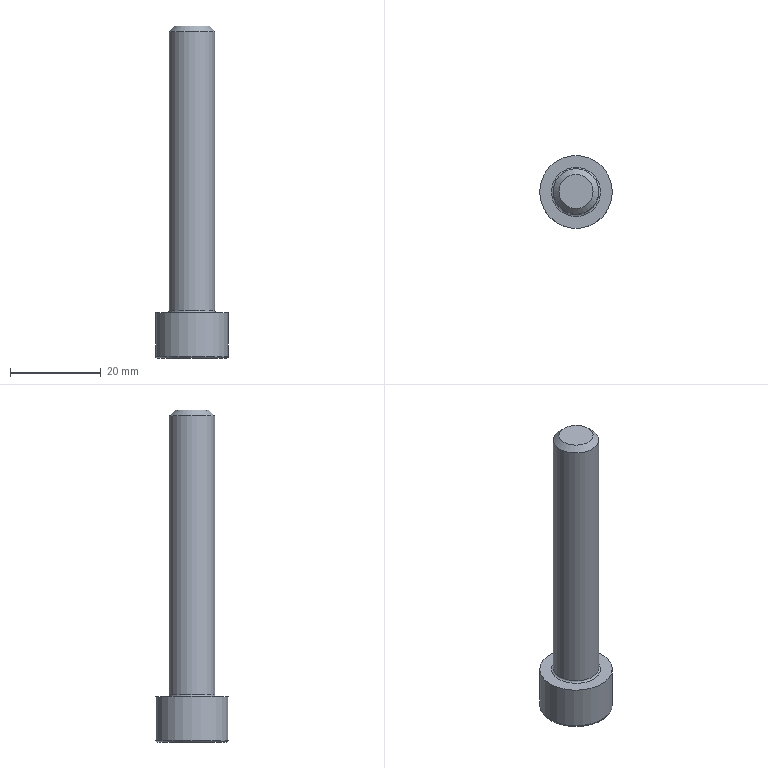Part | STEP file | solid 166 | 1 solid | 15 faces | box 16 x 16 x 73 mm | volume 6658 mm3 | plane 10 | cylinder 2 | torus 2 | cone 1 | commonest cylinder face diameters 10 x1 16 x1